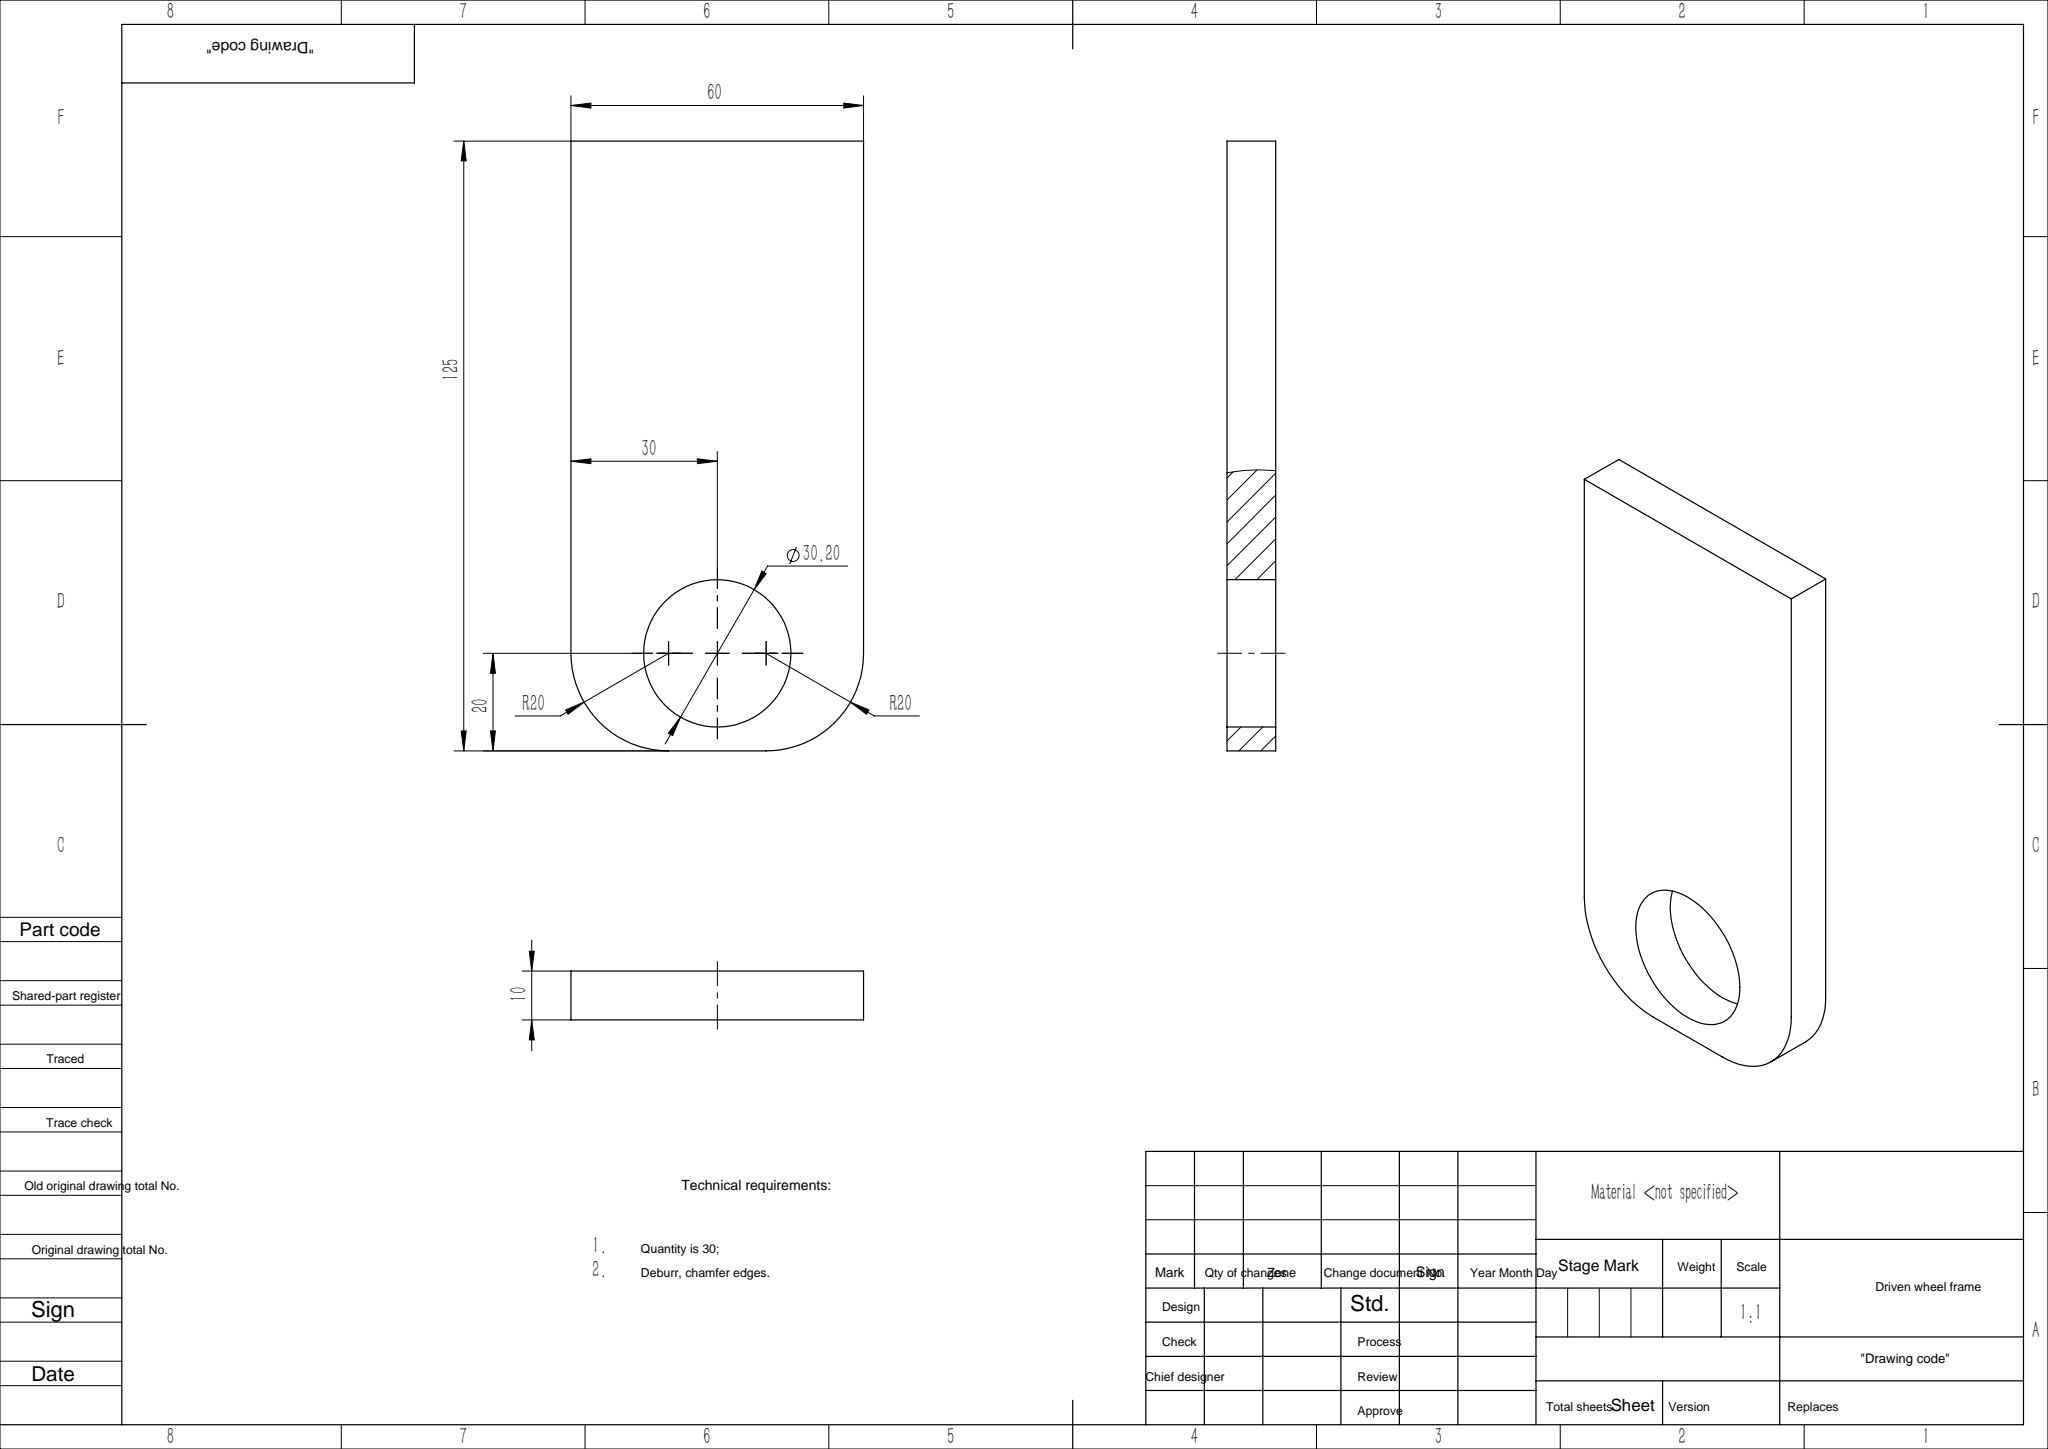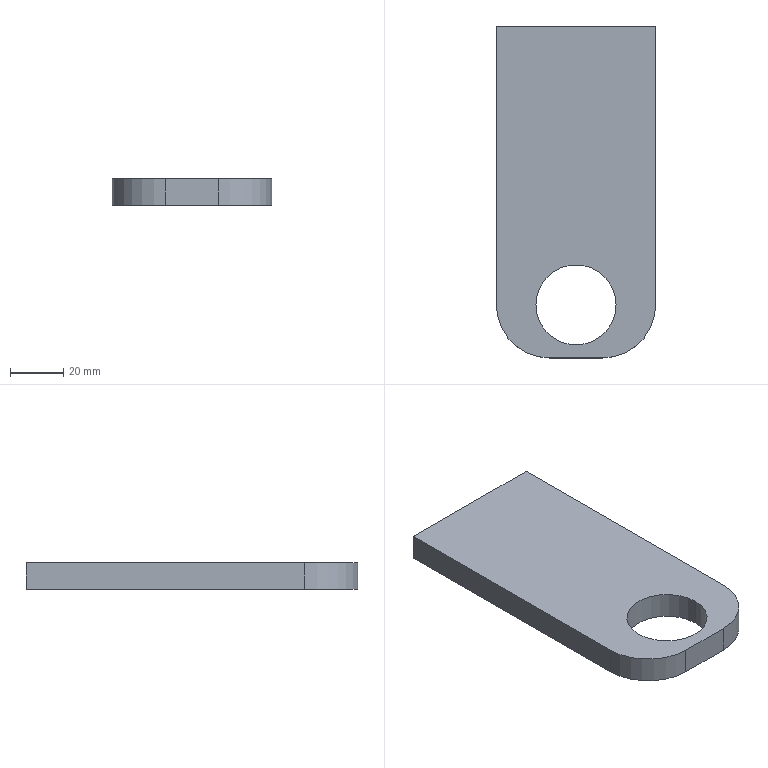Part | SolidWorks | features Extrusion 1, Fillet 1 | 1 solid | 10 faces | box 60 x 125 x 10 mm | volume 66120 mm3 | plane 6 | cylinder 4 | commonest cylinder face diameters 30.2 x2 40 x2
STEP:
#1=CARTESIAN_POINT('',(-15.1,0.,10.));
#2=VERTEX_POINT('',#1);
#3=CARTESIAN_POINT('',(15.1,0.,10.));
#4=VERTEX_POINT('',#3);
#5=CARTESIAN_POINT('',(0.,0.,10.));
#6=DIRECTION('',(0.,0.,1.));
#7=DIRECTION('',(1.,0.,0.));
#8=AXIS2_PLACEMENT_3D('',#5,#6,#7);
#9=CIRCLE('',#8,15.1);
#10=EDGE_CURVE('',#2,#4,#9,.T.);
#11=ORIENTED_EDGE('',*,*,#10,.T.);
#12=CARTESIAN_POINT('',(15.1,0.,0.));
#13=VERTEX_POINT('',#12);
#14=CARTESIAN_POINT('',(15.1,0.,10.));
#15=DIRECTION('',(0.,0.,-1.));
#16=VECTOR('',#15,1000.);
#17=LINE('',#14,#16);
#18=EDGE_CURVE('',#4,#13,#17,.T.);
#19=ORIENTED_EDGE('',*,*,#18,.T.);
#20=CARTESIAN_POINT('',(-15.1,0.,0.));
#21=VERTEX_POINT('',#20);
#22=CARTESIAN_POINT('',(0.,0.,0.));
#23=DIRECTION('',(0.,0.,1.));
#24=DIRECTION('',(1.,0.,0.));
#25=AXIS2_PLACEMENT_3D('',#22,#23,#24);
#26=CIRCLE('',#25,15.1);
#27=EDGE_CURVE('',#21,#13,#26,.T.);
#28=ORIENTED_EDGE('',*,*,#27,.F.);
#29=CARTESIAN_POINT('',(-15.1,0.,10.));
#30=DIRECTION('',(0.,0.,-1.));
#31=VECTOR('',#30,1000.);
#32=LINE('',#29,#31);
#33=EDGE_CURVE('',#2,#21,#32,.T.);
#34=ORIENTED_EDGE('',*,*,#33,.F.);
#35=EDGE_LOOP('',(#11,#19,#28,#34));
#36=FACE_OUTER_BOUND('',#35,.T.);
#37=CARTESIAN_POINT('',(0.,0.,10.));
#38=DIRECTION('',(0.,0.,-1.));
#39=DIRECTION('',(-1.,0.,0.));
#40=AXIS2_PLACEMENT_3D('',#37,#38,#39);
#41=CYLINDRICAL_SURFACE('',#40,15.1);
#42=ADVANCED_FACE('',(#36),#41,.F.);
#43=CARTESIAN_POINT('',(-30.,105.,10.));
#44=VERTEX_POINT('',#43);
#45=CARTESIAN_POINT('',(-30.,0.,10.));
#46=VERTEX_POINT('',#45);
#47=CARTESIAN_POINT('',(-30.,105.,10.));
#48=DIRECTION('',(0.,-1.,0.));
#49=VECTOR('',#48,1000.);
#50=LINE('',#47,#49);
#51=EDGE_CURVE('',#44,#46,#50,.T.);
#52=ORIENTED_EDGE('',*,*,#51,.T.);
#53=CARTESIAN_POINT('',(-10.,-20.,10.));
#54=VERTEX_POINT('',#53);
#55=CARTESIAN_POINT('',(-10.,0.,10.));
#56=DIRECTION('',(0.,0.,1.));
#57=DIRECTION('',(1.,0.,0.));
#58=AXIS2_PLACEMENT_3D('',#55,#56,#57);
#59=CIRCLE('',#58,20.);
#60=EDGE_CURVE('',#46,#54,#59,.T.);
#61=ORIENTED_EDGE('',*,*,#60,.T.);
#62=CARTESIAN_POINT('',(10.,-20.,10.));
#63=VERTEX_POINT('',#62);
#64=CARTESIAN_POINT('',(-30.,-20.,10.));
#65=DIRECTION('',(1.,0.,0.));
#66=VECTOR('',#65,1000.);
#67=LINE('',#64,#66);
#68=EDGE_CURVE('',#54,#63,#67,.T.);
#69=ORIENTED_EDGE('',*,*,#68,.T.);
#70=CARTESIAN_POINT('',(30.,0.,10.));
#71=VERTEX_POINT('',#70);
#72=CARTESIAN_POINT('',(10.,0.,10.));
#73=DIRECTION('',(0.,0.,1.));
#74=DIRECTION('',(1.,0.,0.));
#75=AXIS2_PLACEMENT_3D('',#72,#73,#74);
#76=CIRCLE('',#75,20.);
#77=EDGE_CURVE('',#63,#71,#76,.T.);
#78=ORIENTED_EDGE('',*,*,#77,.T.);
#79=CARTESIAN_POINT('',(30.,105.,10.));
#80=VERTEX_POINT('',#79);
#81=CARTESIAN_POINT('',(30.,105.,10.));
#82=DIRECTION('',(0.,1.,0.));
#83=VECTOR('',#82,1000.);
#84=LINE('',#81,#83);
#85=EDGE_CURVE('',#71,#80,#84,.T.);
#86=ORIENTED_EDGE('',*,*,#85,.T.);
#87=CARTESIAN_POINT('',(-30.,105.,10.));
#88=DIRECTION('',(-1.,0.,0.));
#89=VECTOR('',#88,1000.);
#90=LINE('',#87,#89);
#91=EDGE_CURVE('',#80,#44,#90,.T.);
#92=ORIENTED_EDGE('',*,*,#91,.T.);
#93=EDGE_LOOP('',(#52,#61,#69,#78,#86,#92));
#94=FACE_OUTER_BOUND('',#93,.T.);
#95=ORIENTED_EDGE('',*,*,#10,.F.);
#96=CARTESIAN_POINT('',(0.,0.,10.));
#97=DIRECTION('',(0.,0.,1.));
#98=DIRECTION('',(1.,0.,0.));
#99=AXIS2_PLACEMENT_3D('',#96,#97,#98);
#100=CIRCLE('',#99,15.1);
#101=EDGE_CURVE('',#4,#2,#100,.T.);
#102=ORIENTED_EDGE('',*,*,#101,.F.);
#103=EDGE_LOOP('',(#95,#102));
#104=FACE_BOUND('',#103,.T.);
#105=CARTESIAN_POINT('',(0.,0.,10.));
#106=DIRECTION('',(0.,0.,1.));
#107=DIRECTION('',(1.,0.,0.));
#108=AXIS2_PLACEMENT_3D('',#105,#106,#107);
#109=PLANE('',#108);
#110=ADVANCED_FACE('',(#94,#104),#109,.T.);
#111=CARTESIAN_POINT('',(-10.,-20.,0.));
#112=VERTEX_POINT('',#111);
#113=CARTESIAN_POINT('',(10.,-20.,0.));
#114=VERTEX_POINT('',#113);
#115=CARTESIAN_POINT('',(-30.,-20.,0.));
#116=DIRECTION('',(1.,0.,0.));
#117=VECTOR('',#116,1000.);
#118=LINE('',#115,#117);
#119=EDGE_CURVE('',#112,#114,#118,.T.);
#120=ORIENTED_EDGE('',*,*,#119,.F.);
#121=CARTESIAN_POINT('',(-30.,0.,0.));
#122=VERTEX_POINT('',#121);
#123=CARTESIAN_POINT('',(-10.,0.,0.));
#124=DIRECTION('',(0.,0.,-1.));
#125=DIRECTION('',(1.,0.,0.));
#126=AXIS2_PLACEMENT_3D('',#123,#124,#125);
#127=CIRCLE('',#126,20.);
#128=EDGE_CURVE('',#112,#122,#127,.T.);
#129=ORIENTED_EDGE('',*,*,#128,.T.);
#130=CARTESIAN_POINT('',(-30.,105.,0.));
#131=VERTEX_POINT('',#130);
#132=CARTESIAN_POINT('',(-30.,105.,0.));
#133=DIRECTION('',(0.,-1.,0.));
#134=VECTOR('',#133,1000.);
#135=LINE('',#132,#134);
#136=EDGE_CURVE('',#131,#122,#135,.T.);
#137=ORIENTED_EDGE('',*,*,#136,.F.);
#138=CARTESIAN_POINT('',(30.,105.,0.));
#139=VERTEX_POINT('',#138);
#140=CARTESIAN_POINT('',(-30.,105.,0.));
#141=DIRECTION('',(-1.,0.,0.));
#142=VECTOR('',#141,1000.);
#143=LINE('',#140,#142);
#144=EDGE_CURVE('',#139,#131,#143,.T.);
#145=ORIENTED_EDGE('',*,*,#144,.F.);
#146=CARTESIAN_POINT('',(30.,0.,0.));
#147=VERTEX_POINT('',#146);
#148=CARTESIAN_POINT('',(30.,105.,0.));
#149=DIRECTION('',(0.,1.,0.));
#150=VECTOR('',#149,1000.);
#151=LINE('',#148,#150);
#152=EDGE_CURVE('',#147,#139,#151,.T.);
#153=ORIENTED_EDGE('',*,*,#152,.F.);
#154=CARTESIAN_POINT('',(10.,0.,0.));
#155=DIRECTION('',(0.,0.,-1.));
#156=DIRECTION('',(1.,0.,0.));
#157=AXIS2_PLACEMENT_3D('',#154,#155,#156);
#158=CIRCLE('',#157,20.);
#159=EDGE_CURVE('',#147,#114,#158,.T.);
#160=ORIENTED_EDGE('',*,*,#159,.T.);
#161=EDGE_LOOP('',(#120,#129,#137,#145,#153,#160));
#162=FACE_OUTER_BOUND('',#161,.T.);
#163=ORIENTED_EDGE('',*,*,#27,.T.);
#164=CARTESIAN_POINT('',(0.,0.,0.));
#165=DIRECTION('',(0.,0.,1.));
#166=DIRECTION('',(1.,0.,0.));
#167=AXIS2_PLACEMENT_3D('',#164,#165,#166);
#168=CIRCLE('',#167,15.1);
#169=EDGE_CURVE('',#13,#21,#168,.T.);
#170=ORIENTED_EDGE('',*,*,#169,.T.);
#171=EDGE_LOOP('',(#163,#170));
#172=FACE_BOUND('',#171,.T.);
#173=CARTESIAN_POINT('',(0.,0.,0.));
#174=DIRECTION('',(0.,0.,1.));
#175=DIRECTION('',(1.,0.,0.));
#176=AXIS2_PLACEMENT_3D('',#173,#174,#175);
#177=PLANE('',#176);
#178=ADVANCED_FACE('',(#162,#172),#177,.F.);
#179=ORIENTED_EDGE('',*,*,#136,.T.);
#180=CARTESIAN_POINT('',(-30.,0.,10.));
#181=DIRECTION('',(0.,0.,1.));
#182=VECTOR('',#181,1000.);
#183=LINE('',#180,#182);
#184=EDGE_CURVE('',#122,#46,#183,.T.);
#185=ORIENTED_EDGE('',*,*,#184,.T.);
#186=ORIENTED_EDGE('',*,*,#51,.F.);
#187=CARTESIAN_POINT('',(-30.,105.,10.));
#188=DIRECTION('',(0.,0.,-1.));
#189=VECTOR('',#188,1000.);
#190=LINE('',#187,#189);
#191=EDGE_CURVE('',#44,#131,#190,.T.);
#192=ORIENTED_EDGE('',*,*,#191,.T.);
#193=EDGE_LOOP('',(#179,#185,#186,#192));
#194=FACE_OUTER_BOUND('',#193,.T.);
#195=CARTESIAN_POINT('',(-30.,105.,10.));
#196=DIRECTION('',(1.,0.,0.));
#197=DIRECTION('',(0.,1.,0.));
#198=AXIS2_PLACEMENT_3D('',#195,#196,#197);
#199=PLANE('',#198);
#200=ADVANCED_FACE('',(#194),#199,.F.);
#201=ORIENTED_EDGE('',*,*,#68,.F.);
#202=CARTESIAN_POINT('',(-10.,-20.,10.));
#203=DIRECTION('',(0.,0.,-1.));
#204=VECTOR('',#203,1000.);
#205=LINE('',#202,#204);
#206=EDGE_CURVE('',#54,#112,#205,.T.);
#207=ORIENTED_EDGE('',*,*,#206,.T.);
#208=ORIENTED_EDGE('',*,*,#119,.T.);
#209=CARTESIAN_POINT('',(10.,-20.,10.));
#210=DIRECTION('',(0.,0.,1.));
#211=VECTOR('',#210,1000.);
#212=LINE('',#209,#211);
#213=EDGE_CURVE('',#114,#63,#212,.T.);
#214=ORIENTED_EDGE('',*,*,#213,.T.);
#215=EDGE_LOOP('',(#201,#207,#208,#214));
#216=FACE_OUTER_BOUND('',#215,.T.);
#217=CARTESIAN_POINT('',(-30.,-20.,10.));
#218=DIRECTION('',(0.,1.,0.));
#219=DIRECTION('',(0.,0.,1.));
#220=AXIS2_PLACEMENT_3D('',#217,#218,#219);
#221=PLANE('',#220);
#222=ADVANCED_FACE('',(#216),#221,.F.);
#223=ORIENTED_EDGE('',*,*,#85,.F.);
#224=CARTESIAN_POINT('',(30.,0.,10.));
#225=DIRECTION('',(0.,0.,-1.));
#226=VECTOR('',#225,1000.);
#227=LINE('',#224,#226);
#228=EDGE_CURVE('',#71,#147,#227,.T.);
#229=ORIENTED_EDGE('',*,*,#228,.T.);
#230=ORIENTED_EDGE('',*,*,#152,.T.);
#231=CARTESIAN_POINT('',(30.,105.,10.));
#232=DIRECTION('',(0.,0.,-1.));
#233=VECTOR('',#232,1000.);
#234=LINE('',#231,#233);
#235=EDGE_CURVE('',#80,#139,#234,.T.);
#236=ORIENTED_EDGE('',*,*,#235,.F.);
#237=EDGE_LOOP('',(#223,#229,#230,#236));
#238=FACE_OUTER_BOUND('',#237,.T.);
#239=CARTESIAN_POINT('',(30.,105.,10.));
#240=DIRECTION('',(-1.,0.,0.));
#241=DIRECTION('',(0.,-1.,0.));
#242=AXIS2_PLACEMENT_3D('',#239,#240,#241);
#243=PLANE('',#242);
#244=ADVANCED_FACE('',(#238),#243,.F.);
#245=ORIENTED_EDGE('',*,*,#144,.T.);
#246=ORIENTED_EDGE('',*,*,#191,.F.);
#247=ORIENTED_EDGE('',*,*,#91,.F.);
#248=ORIENTED_EDGE('',*,*,#235,.T.);
#249=EDGE_LOOP('',(#245,#246,#247,#248));
#250=FACE_OUTER_BOUND('',#249,.T.);
#251=CARTESIAN_POINT('',(-30.,105.,10.));
#252=DIRECTION('',(0.,-1.,0.));
#253=DIRECTION('',(1.,0.,0.));
#254=AXIS2_PLACEMENT_3D('',#251,#252,#253);
#255=PLANE('',#254);
#256=ADVANCED_FACE('',(#250),#255,.F.);
#257=ORIENTED_EDGE('',*,*,#18,.F.);
#258=ORIENTED_EDGE('',*,*,#101,.T.);
#259=ORIENTED_EDGE('',*,*,#33,.T.);
#260=ORIENTED_EDGE('',*,*,#169,.F.);
#261=EDGE_LOOP('',(#257,#258,#259,#260));
#262=FACE_OUTER_BOUND('',#261,.T.);
#263=CARTESIAN_POINT('',(0.,0.,10.));
#264=DIRECTION('',(0.,0.,-1.));
#265=DIRECTION('',(-1.,0.,0.));
#266=AXIS2_PLACEMENT_3D('',#263,#264,#265);
#267=CYLINDRICAL_SURFACE('',#266,15.1);
#268=ADVANCED_FACE('',(#262),#267,.F.);
#269=ORIENTED_EDGE('',*,*,#60,.F.);
#270=ORIENTED_EDGE('',*,*,#184,.F.);
#271=ORIENTED_EDGE('',*,*,#128,.F.);
#272=ORIENTED_EDGE('',*,*,#206,.F.);
#273=EDGE_LOOP('',(#269,#270,#271,#272));
#274=FACE_OUTER_BOUND('',#273,.T.);
#275=CARTESIAN_POINT('',(-10.,0.,10.));
#276=DIRECTION('',(0.,0.,-1.));
#277=DIRECTION('',(-1.,0.,0.));
#278=AXIS2_PLACEMENT_3D('',#275,#276,#277);
#279=CYLINDRICAL_SURFACE('',#278,20.);
#280=ADVANCED_FACE('',(#274),#279,.T.);
#281=ORIENTED_EDGE('',*,*,#77,.F.);
#282=ORIENTED_EDGE('',*,*,#213,.F.);
#283=ORIENTED_EDGE('',*,*,#159,.F.);
#284=ORIENTED_EDGE('',*,*,#228,.F.);
#285=EDGE_LOOP('',(#281,#282,#283,#284));
#286=FACE_OUTER_BOUND('',#285,.T.);
#287=CARTESIAN_POINT('',(10.,0.,10.));
#288=DIRECTION('',(0.,0.,-1.));
#289=DIRECTION('',(-1.,0.,0.));
#290=AXIS2_PLACEMENT_3D('',#287,#288,#289);
#291=CYLINDRICAL_SURFACE('',#290,20.);
#292=ADVANCED_FACE('',(#286),#291,.T.);
#293=CLOSED_SHELL('',(#42,#110,#178,#200,#222,#244,#256,#268,#280,#292));
#294=MANIFOLD_SOLID_BREP('',#293);
#295=CARTESIAN_POINT('',(0.,0.,0.));
#296=DIRECTION('',(0.,0.,1.));
#297=DIRECTION('',(1.,0.,0.));
#298=AXIS2_PLACEMENT_3D('',#295,#296,#297);
#299=(LENGTH_UNIT()NAMED_UNIT(*)SI_UNIT(.MILLI.,.METRE.));
#300=UNCERTAINTY_MEASURE_WITH_UNIT(LENGTH_MEASURE(0.00001),#299,'','');
#301=(NAMED_UNIT(*)PLANE_ANGLE_UNIT()SI_UNIT($,.RADIAN.));
#302=(NAMED_UNIT(*)SI_UNIT($,.STERADIAN.)SOLID_ANGLE_UNIT());
#303=(GEOMETRIC_REPRESENTATION_CONTEXT(3)GLOBAL_UNCERTAINTY_ASSIGNED_CONTEXT((#300))GLOBAL_UNIT_ASSIGNED_CONTEXT((#299,#301,#302))REPRESENTATION_CONTEXT('',''));
#304=ADVANCED_BREP_SHAPE_REPRESENTATION('',(#294,#298),#303);